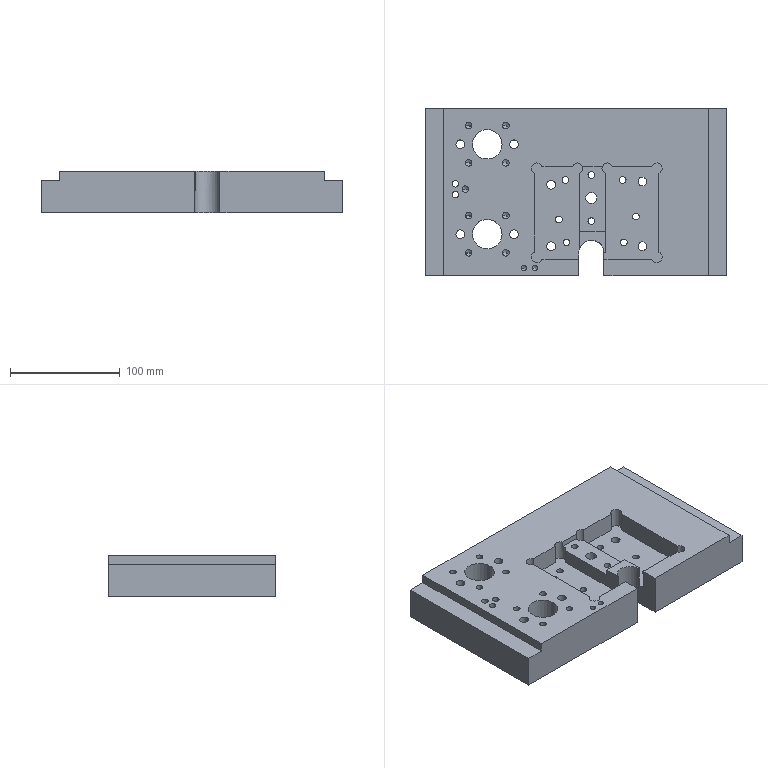Part | 1 solid | 125 faces | box 275.4 x 153 x 38 mm | volume 1312247 mm3 | cylinder 74 | plane 27 | cone 24 | commonest cylinder face diameters 6 x38 8 x16 10 x9 5 x4 27 x4 12 x2